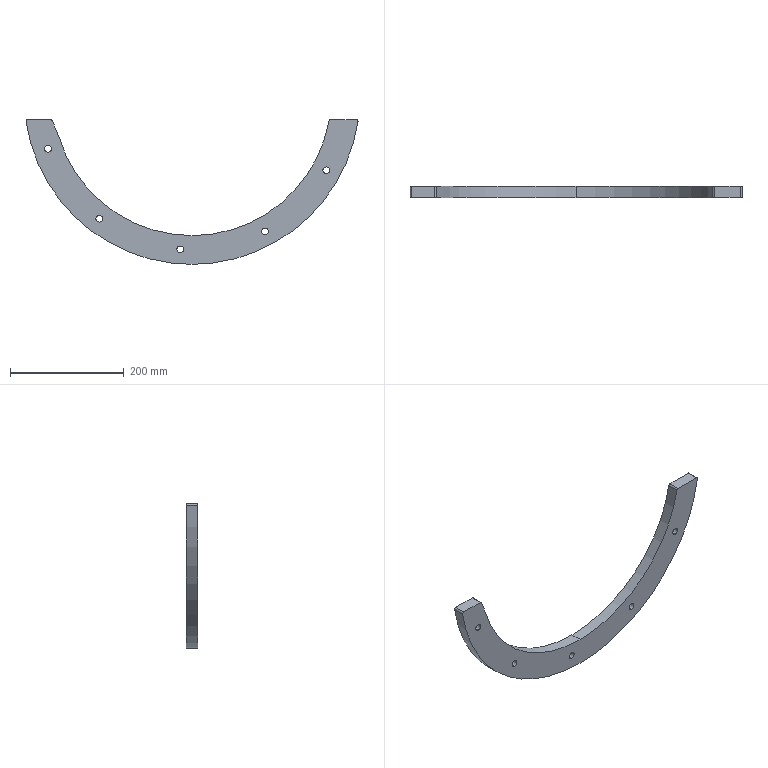Part | SolidWorks | features BaseBody 1 | 1 solid | 23 faces | box 584.886 x 20 x 255 mm | volume 765940 mm3 | cylinder 18 | plane 5 | commonest cylinder face diameters 12 x10 6 x4 490 x2 591.455 x2
STEP:
#1=CARTESIAN_POINT('',(-292.409,20.,-44.175));
#2=VERTEX_POINT('',#1);
#3=CARTESIAN_POINT('',(0.,20.,-295.727));
#4=VERTEX_POINT('',#3);
#5=CARTESIAN_POINT('',(0.,20.,0.));
#6=DIRECTION('',(0.,-1.,0.));
#7=DIRECTION('',(0.,0.,-1.));
#8=AXIS2_PLACEMENT_3D('',#5,#6,#7);
#9=CIRCLE('',#8,295.727);
#10=EDGE_CURVE('',#2,#4,#9,.T.);
#11=ORIENTED_EDGE('',*,*,#10,.T.);
#12=CARTESIAN_POINT('',(0.,0.,-295.727));
#13=VERTEX_POINT('',#12);
#14=CARTESIAN_POINT('',(0.,20.,-295.727));
#15=DIRECTION('',(0.,-1.,0.));
#16=VECTOR('',#15,1000.);
#17=LINE('',#14,#16);
#18=EDGE_CURVE('',#4,#13,#17,.T.);
#19=ORIENTED_EDGE('',*,*,#18,.T.);
#20=CARTESIAN_POINT('',(-292.409,0.,-44.175));
#21=VERTEX_POINT('',#20);
#22=CARTESIAN_POINT('',(0.,0.,0.));
#23=DIRECTION('',(0.,1.,0.));
#24=DIRECTION('',(0.,0.,-1.));
#25=AXIS2_PLACEMENT_3D('',#22,#23,#24);
#26=CIRCLE('',#25,295.727);
#27=EDGE_CURVE('',#13,#21,#26,.T.);
#28=ORIENTED_EDGE('',*,*,#27,.T.);
#29=CARTESIAN_POINT('',(-292.409,20.,-44.175));
#30=DIRECTION('',(0.,-1.,0.));
#31=VECTOR('',#30,1000.);
#32=LINE('',#29,#31);
#33=EDGE_CURVE('',#2,#21,#32,.T.);
#34=ORIENTED_EDGE('',*,*,#33,.F.);
#35=EDGE_LOOP('',(#11,#19,#28,#34));
#36=FACE_OUTER_BOUND('',#35,.T.);
#37=CARTESIAN_POINT('',(0.,20.,0.));
#38=DIRECTION('',(0.,-1.,0.));
#39=DIRECTION('',(0.,0.,-1.));
#40=AXIS2_PLACEMENT_3D('',#37,#38,#39);
#41=CYLINDRICAL_SURFACE('',#40,295.727);
#42=ADVANCED_FACE('',(#36),#41,.T.);
#43=CARTESIAN_POINT('',(0.,20.,-245.));
#44=VERTEX_POINT('',#43);
#45=CARTESIAN_POINT('',(241.162,20.,-43.198));
#46=VERTEX_POINT('',#45);
#47=CARTESIAN_POINT('',(0.,20.,0.));
#48=DIRECTION('',(0.,-1.,0.));
#49=DIRECTION('',(0.,0.,-1.));
#50=AXIS2_PLACEMENT_3D('',#47,#48,#49);
#51=CIRCLE('',#50,245.);
#52=EDGE_CURVE('',#44,#46,#51,.T.);
#53=ORIENTED_EDGE('',*,*,#52,.F.);
#54=CARTESIAN_POINT('',(0.,0.,-245.));
#55=VERTEX_POINT('',#54);
#56=CARTESIAN_POINT('',(0.,20.,-245.));
#57=DIRECTION('',(0.,-1.,0.));
#58=VECTOR('',#57,1000.);
#59=LINE('',#56,#58);
#60=EDGE_CURVE('',#44,#55,#59,.T.);
#61=ORIENTED_EDGE('',*,*,#60,.T.);
#62=CARTESIAN_POINT('',(241.162,0.,-43.198));
#63=VERTEX_POINT('',#62);
#64=CARTESIAN_POINT('',(0.,0.,0.));
#65=DIRECTION('',(0.,-1.,0.));
#66=DIRECTION('',(0.,0.,-1.));
#67=AXIS2_PLACEMENT_3D('',#64,#65,#66);
#68=CIRCLE('',#67,245.);
#69=EDGE_CURVE('',#55,#63,#68,.T.);
#70=ORIENTED_EDGE('',*,*,#69,.T.);
#71=CARTESIAN_POINT('',(241.162,20.,-43.198));
#72=DIRECTION('',(0.,-1.,0.));
#73=VECTOR('',#72,1000.);
#74=LINE('',#71,#73);
#75=EDGE_CURVE('',#46,#63,#74,.T.);
#76=ORIENTED_EDGE('',*,*,#75,.F.);
#77=EDGE_LOOP('',(#53,#61,#70,#76));
#78=FACE_OUTER_BOUND('',#77,.T.);
#79=CARTESIAN_POINT('',(0.,20.,0.));
#80=DIRECTION('',(0.,-1.,0.));
#81=DIRECTION('',(0.,0.,-1.));
#82=AXIS2_PLACEMENT_3D('',#79,#80,#81);
#83=CYLINDRICAL_SURFACE('',#82,245.);
#84=ADVANCED_FACE('',(#78),#83,.F.);
#85=CARTESIAN_POINT('',(-253.717,0.,-86.345));
#86=VERTEX_POINT('',#85);
#87=CARTESIAN_POINT('',(-253.717,0.,-98.345));
#88=VERTEX_POINT('',#87);
#89=CARTESIAN_POINT('',(-253.717,0.,-92.345));
#90=DIRECTION('',(0.,-1.,0.));
#91=DIRECTION('',(0.,0.,1.));
#92=AXIS2_PLACEMENT_3D('',#89,#90,#91);
#93=CIRCLE('',#92,6.);
#94=EDGE_CURVE('',#86,#88,#93,.T.);
#95=ORIENTED_EDGE('',*,*,#94,.T.);
#96=CARTESIAN_POINT('',(-253.717,20.,-98.345));
#97=VERTEX_POINT('',#96);
#98=CARTESIAN_POINT('',(-253.717,20.,-98.345));
#99=DIRECTION('',(0.,1.,0.));
#100=VECTOR('',#99,1000.);
#101=LINE('',#98,#100);
#102=EDGE_CURVE('',#88,#97,#101,.T.);
#103=ORIENTED_EDGE('',*,*,#102,.T.);
#104=CARTESIAN_POINT('',(-253.717,20.,-86.345));
#105=VERTEX_POINT('',#104);
#106=CARTESIAN_POINT('',(-253.717,20.,-92.345));
#107=DIRECTION('',(0.,-1.,0.));
#108=DIRECTION('',(0.,0.,1.));
#109=AXIS2_PLACEMENT_3D('',#106,#107,#108);
#110=CIRCLE('',#109,6.);
#111=EDGE_CURVE('',#105,#97,#110,.T.);
#112=ORIENTED_EDGE('',*,*,#111,.F.);
#113=CARTESIAN_POINT('',(-253.717,20.,-86.345));
#114=DIRECTION('',(0.,1.,0.));
#115=VECTOR('',#114,1000.);
#116=LINE('',#113,#115);
#117=EDGE_CURVE('',#86,#105,#116,.T.);
#118=ORIENTED_EDGE('',*,*,#117,.F.);
#119=EDGE_LOOP('',(#95,#103,#112,#118));
#120=FACE_OUTER_BOUND('',#119,.T.);
#121=CARTESIAN_POINT('',(-253.717,20.,-92.345));
#122=DIRECTION('',(0.,1.,0.));
#123=DIRECTION('',(0.,0.,1.));
#124=AXIS2_PLACEMENT_3D('',#121,#122,#123);
#125=CYLINDRICAL_SURFACE('',#124,6.);
#126=ADVANCED_FACE('',(#120),#125,.F.);
#127=CARTESIAN_POINT('',(236.708,0.,-124.148));
#128=VERTEX_POINT('',#127);
#129=CARTESIAN_POINT('',(236.708,0.,-136.148));
#130=VERTEX_POINT('',#129);
#131=CARTESIAN_POINT('',(236.708,0.,-130.148));
#132=DIRECTION('',(0.,-1.,0.));
#133=DIRECTION('',(0.,0.,1.));
#134=AXIS2_PLACEMENT_3D('',#131,#132,#133);
#135=CIRCLE('',#134,6.);
#136=EDGE_CURVE('',#128,#130,#135,.T.);
#137=ORIENTED_EDGE('',*,*,#136,.T.);
#138=CARTESIAN_POINT('',(236.708,20.,-136.148));
#139=VERTEX_POINT('',#138);
#140=CARTESIAN_POINT('',(236.708,20.,-136.148));
#141=DIRECTION('',(0.,1.,0.));
#142=VECTOR('',#141,1000.);
#143=LINE('',#140,#142);
#144=EDGE_CURVE('',#130,#139,#143,.T.);
#145=ORIENTED_EDGE('',*,*,#144,.T.);
#146=CARTESIAN_POINT('',(236.708,20.,-124.148));
#147=VERTEX_POINT('',#146);
#148=CARTESIAN_POINT('',(236.708,20.,-130.148));
#149=DIRECTION('',(0.,-1.,0.));
#150=DIRECTION('',(0.,0.,1.));
#151=AXIS2_PLACEMENT_3D('',#148,#149,#150);
#152=CIRCLE('',#151,6.);
#153=EDGE_CURVE('',#147,#139,#152,.T.);
#154=ORIENTED_EDGE('',*,*,#153,.F.);
#155=CARTESIAN_POINT('',(236.708,20.,-124.148));
#156=DIRECTION('',(0.,1.,0.));
#157=VECTOR('',#156,1000.);
#158=LINE('',#155,#157);
#159=EDGE_CURVE('',#128,#147,#158,.T.);
#160=ORIENTED_EDGE('',*,*,#159,.F.);
#161=EDGE_LOOP('',(#137,#145,#154,#160));
#162=FACE_OUTER_BOUND('',#161,.T.);
#163=CARTESIAN_POINT('',(236.708,20.,-130.148));
#164=DIRECTION('',(0.,1.,0.));
#165=DIRECTION('',(0.,0.,1.));
#166=AXIS2_PLACEMENT_3D('',#163,#164,#165);
#167=CYLINDRICAL_SURFACE('',#166,6.);
#168=ADVANCED_FACE('',(#162),#167,.F.);
#169=CARTESIAN_POINT('',(128.503,0.,-231.651));
#170=VERTEX_POINT('',#169);
#171=CARTESIAN_POINT('',(128.503,0.,-243.651));
#172=VERTEX_POINT('',#171);
#173=CARTESIAN_POINT('',(128.503,0.,-237.651));
#174=DIRECTION('',(0.,-1.,0.));
#175=DIRECTION('',(0.,0.,1.));
#176=AXIS2_PLACEMENT_3D('',#173,#174,#175);
#177=CIRCLE('',#176,6.);
#178=EDGE_CURVE('',#170,#172,#177,.T.);
#179=ORIENTED_EDGE('',*,*,#178,.T.);
#180=CARTESIAN_POINT('',(128.503,20.,-243.651));
#181=VERTEX_POINT('',#180);
#182=CARTESIAN_POINT('',(128.503,20.,-243.651));
#183=DIRECTION('',(0.,1.,0.));
#184=VECTOR('',#183,1000.);
#185=LINE('',#182,#184);
#186=EDGE_CURVE('',#172,#181,#185,.T.);
#187=ORIENTED_EDGE('',*,*,#186,.T.);
#188=CARTESIAN_POINT('',(128.503,20.,-231.651));
#189=VERTEX_POINT('',#188);
#190=CARTESIAN_POINT('',(128.503,20.,-237.651));
#191=DIRECTION('',(0.,-1.,0.));
#192=DIRECTION('',(0.,0.,1.));
#193=AXIS2_PLACEMENT_3D('',#190,#191,#192);
#194=CIRCLE('',#193,6.);
#195=EDGE_CURVE('',#189,#181,#194,.T.);
#196=ORIENTED_EDGE('',*,*,#195,.F.);
#197=CARTESIAN_POINT('',(128.503,20.,-231.651));
#198=DIRECTION('',(0.,1.,0.));
#199=VECTOR('',#198,1000.);
#200=LINE('',#197,#199);
#201=EDGE_CURVE('',#170,#189,#200,.T.);
#202=ORIENTED_EDGE('',*,*,#201,.F.);
#203=EDGE_LOOP('',(#179,#187,#196,#202));
#204=FACE_OUTER_BOUND('',#203,.T.);
#205=CARTESIAN_POINT('',(128.503,20.,-237.651));
#206=DIRECTION('',(0.,1.,0.));
#207=DIRECTION('',(0.,0.,1.));
#208=AXIS2_PLACEMENT_3D('',#205,#206,#207);
#209=CYLINDRICAL_SURFACE('',#208,6.);
#210=ADVANCED_FACE('',(#204),#209,.F.);
#211=CARTESIAN_POINT('',(-20.692,0.,-263.361));
#212=VERTEX_POINT('',#211);
#213=CARTESIAN_POINT('',(-20.692,0.,-275.361));
#214=VERTEX_POINT('',#213);
#215=CARTESIAN_POINT('',(-20.692,0.,-269.361));
#216=DIRECTION('',(0.,-1.,0.));
#217=DIRECTION('',(0.,0.,1.));
#218=AXIS2_PLACEMENT_3D('',#215,#216,#217);
#219=CIRCLE('',#218,6.);
#220=EDGE_CURVE('',#212,#214,#219,.T.);
#221=ORIENTED_EDGE('',*,*,#220,.T.);
#222=CARTESIAN_POINT('',(-20.692,20.,-275.361));
#223=VERTEX_POINT('',#222);
#224=CARTESIAN_POINT('',(-20.692,20.,-275.361));
#225=DIRECTION('',(0.,1.,0.));
#226=VECTOR('',#225,1000.);
#227=LINE('',#224,#226);
#228=EDGE_CURVE('',#214,#223,#227,.T.);
#229=ORIENTED_EDGE('',*,*,#228,.T.);
#230=CARTESIAN_POINT('',(-20.692,20.,-263.361));
#231=VERTEX_POINT('',#230);
#232=CARTESIAN_POINT('',(-20.692,20.,-269.361));
#233=DIRECTION('',(0.,-1.,0.));
#234=DIRECTION('',(0.,0.,1.));
#235=AXIS2_PLACEMENT_3D('',#232,#233,#234);
#236=CIRCLE('',#235,6.);
#237=EDGE_CURVE('',#231,#223,#236,.T.);
#238=ORIENTED_EDGE('',*,*,#237,.F.);
#239=CARTESIAN_POINT('',(-20.692,20.,-263.361));
#240=DIRECTION('',(0.,1.,0.));
#241=VECTOR('',#240,1000.);
#242=LINE('',#239,#241);
#243=EDGE_CURVE('',#212,#231,#242,.T.);
#244=ORIENTED_EDGE('',*,*,#243,.F.);
#245=EDGE_LOOP('',(#221,#229,#238,#244));
#246=FACE_OUTER_BOUND('',#245,.T.);
#247=CARTESIAN_POINT('',(-20.692,20.,-269.361));
#248=DIRECTION('',(0.,1.,0.));
#249=DIRECTION('',(0.,0.,1.));
#250=AXIS2_PLACEMENT_3D('',#247,#248,#249);
#251=CYLINDRICAL_SURFACE('',#250,6.);
#252=ADVANCED_FACE('',(#246),#251,.F.);
#253=CARTESIAN_POINT('',(-163.266,0.,-209.161));
#254=VERTEX_POINT('',#253);
#255=CARTESIAN_POINT('',(-163.266,0.,-221.161));
#256=VERTEX_POINT('',#255);
#257=CARTESIAN_POINT('',(-163.266,0.,-215.161));
#258=DIRECTION('',(0.,-1.,0.));
#259=DIRECTION('',(0.,0.,1.));
#260=AXIS2_PLACEMENT_3D('',#257,#258,#259);
#261=CIRCLE('',#260,6.);
#262=EDGE_CURVE('',#254,#256,#261,.T.);
#263=ORIENTED_EDGE('',*,*,#262,.T.);
#264=CARTESIAN_POINT('',(-163.266,20.,-221.161));
#265=VERTEX_POINT('',#264);
#266=CARTESIAN_POINT('',(-163.266,20.,-221.161));
#267=DIRECTION('',(0.,1.,0.));
#268=VECTOR('',#267,1000.);
#269=LINE('',#266,#268);
#270=EDGE_CURVE('',#256,#265,#269,.T.);
#271=ORIENTED_EDGE('',*,*,#270,.T.);
#272=CARTESIAN_POINT('',(-163.266,20.,-209.161));
#273=VERTEX_POINT('',#272);
#274=CARTESIAN_POINT('',(-163.266,20.,-215.161));
#275=DIRECTION('',(0.,-1.,0.));
#276=DIRECTION('',(0.,0.,1.));
#277=AXIS2_PLACEMENT_3D('',#274,#275,#276);
#278=CIRCLE('',#277,6.);
#279=EDGE_CURVE('',#273,#265,#278,.T.);
#280=ORIENTED_EDGE('',*,*,#279,.F.);
#281=CARTESIAN_POINT('',(-163.266,20.,-209.161));
#282=DIRECTION('',(0.,1.,0.));
#283=VECTOR('',#282,1000.);
#284=LINE('',#281,#283);
#285=EDGE_CURVE('',#254,#273,#284,.T.);
#286=ORIENTED_EDGE('',*,*,#285,.F.);
#287=EDGE_LOOP('',(#263,#271,#280,#286));
#288=FACE_OUTER_BOUND('',#287,.T.);
#289=CARTESIAN_POINT('',(-163.266,20.,-215.161));
#290=DIRECTION('',(0.,1.,0.));
#291=DIRECTION('',(0.,0.,1.));
#292=AXIS2_PLACEMENT_3D('',#289,#290,#291);
#293=CYLINDRICAL_SURFACE('',#292,6.);
#294=ADVANCED_FACE('',(#288),#293,.F.);
#295=CARTESIAN_POINT('',(289.443,0.,-40.727));
#296=VERTEX_POINT('',#295);
#297=CARTESIAN_POINT('',(292.409,0.,-44.175));
#298=VERTEX_POINT('',#297);
#299=CARTESIAN_POINT('',(289.443,0.,-43.727));
#300=DIRECTION('',(0.,1.,0.));
#301=DIRECTION('',(0.,0.,-1.));
#302=AXIS2_PLACEMENT_3D('',#299,#300,#301);
#303=CIRCLE('',#302,3.);
#304=EDGE_CURVE('',#296,#298,#303,.T.);
#305=ORIENTED_EDGE('',*,*,#304,.F.);
#306=CARTESIAN_POINT('',(244.115,0.,-40.727));
#307=VERTEX_POINT('',#306);
#308=CARTESIAN_POINT('',(0.,0.,-40.727));
#309=DIRECTION('',(1.,0.,0.));
#310=VECTOR('',#309,1000.);
#311=LINE('',#308,#310);
#312=EDGE_CURVE('',#307,#296,#311,.T.);
#313=ORIENTED_EDGE('',*,*,#312,.F.);
#314=CARTESIAN_POINT('',(244.115,0.,-43.727));
#315=DIRECTION('',(0.,1.,0.));
#316=DIRECTION('',(0.,0.,-1.));
#317=AXIS2_PLACEMENT_3D('',#314,#315,#316);
#318=CIRCLE('',#317,3.);
#319=EDGE_CURVE('',#63,#307,#318,.T.);
#320=ORIENTED_EDGE('',*,*,#319,.F.);
#321=ORIENTED_EDGE('',*,*,#69,.F.);
#322=CARTESIAN_POINT('',(-234.569,0.,-70.727));
#323=VERTEX_POINT('',#322);
#324=CARTESIAN_POINT('',(0.,0.,0.));
#325=DIRECTION('',(0.,-1.,0.));
#326=DIRECTION('',(0.,0.,-1.));
#327=AXIS2_PLACEMENT_3D('',#324,#325,#326);
#328=CIRCLE('',#327,245.);
#329=EDGE_CURVE('',#323,#55,#328,.T.);
#330=ORIENTED_EDGE('',*,*,#329,.F.);
#331=CARTESIAN_POINT('',(-246.065,0.,-42.592));
#332=VERTEX_POINT('',#331);
#333=CARTESIAN_POINT('',(-246.065,0.,-42.592));
#334=DIRECTION('',(0.3783,0.,-0.9257));
#335=VECTOR('',#334,1000.);
#336=LINE('',#333,#335);
#337=EDGE_CURVE('',#332,#323,#336,.T.);
#338=ORIENTED_EDGE('',*,*,#337,.F.);
#339=CARTESIAN_POINT('',(-248.843,0.,-40.727));
#340=VERTEX_POINT('',#339);
#341=CARTESIAN_POINT('',(-248.843,0.,-43.727));
#342=DIRECTION('',(0.,1.,0.));
#343=DIRECTION('',(0.,0.,-1.));
#344=AXIS2_PLACEMENT_3D('',#341,#342,#343);
#345=CIRCLE('',#344,3.);
#346=EDGE_CURVE('',#340,#332,#345,.T.);
#347=ORIENTED_EDGE('',*,*,#346,.F.);
#348=CARTESIAN_POINT('',(-289.443,0.,-40.727));
#349=VERTEX_POINT('',#348);
#350=CARTESIAN_POINT('',(0.,0.,-40.727));
#351=DIRECTION('',(1.,0.,0.));
#352=VECTOR('',#351,1000.);
#353=LINE('',#350,#352);
#354=EDGE_CURVE('',#349,#340,#353,.T.);
#355=ORIENTED_EDGE('',*,*,#354,.F.);
#356=CARTESIAN_POINT('',(-289.443,0.,-43.727));
#357=DIRECTION('',(0.,1.,0.));
#358=DIRECTION('',(0.,0.,-1.));
#359=AXIS2_PLACEMENT_3D('',#356,#357,#358);
#360=CIRCLE('',#359,3.);
#361=EDGE_CURVE('',#21,#349,#360,.T.);
#362=ORIENTED_EDGE('',*,*,#361,.F.);
#363=ORIENTED_EDGE('',*,*,#27,.F.);
#364=CARTESIAN_POINT('',(0.,0.,0.));
#365=DIRECTION('',(0.,1.,0.));
#366=DIRECTION('',(0.,0.,-1.));
#367=AXIS2_PLACEMENT_3D('',#364,#365,#366);
#368=CIRCLE('',#367,295.727);
#369=EDGE_CURVE('',#298,#13,#368,.T.);
#370=ORIENTED_EDGE('',*,*,#369,.F.);
#371=EDGE_LOOP('',(#305,#313,#320,#321,#330,#338,#347,#355,#362,#363,#370));
#372=FACE_OUTER_BOUND('',#371,.T.);
#373=ORIENTED_EDGE('',*,*,#94,.F.);
#374=CARTESIAN_POINT('',(-253.717,0.,-92.345));
#375=DIRECTION('',(0.,-1.,0.));
#376=DIRECTION('',(0.,0.,1.));
#377=AXIS2_PLACEMENT_3D('',#374,#375,#376);
#378=CIRCLE('',#377,6.);
#379=EDGE_CURVE('',#88,#86,#378,.T.);
#380=ORIENTED_EDGE('',*,*,#379,.F.);
#381=EDGE_LOOP('',(#373,#380));
#382=FACE_BOUND('',#381,.T.);
#383=ORIENTED_EDGE('',*,*,#136,.F.);
#384=CARTESIAN_POINT('',(236.708,0.,-130.148));
#385=DIRECTION('',(0.,-1.,0.));
#386=DIRECTION('',(0.,0.,1.));
#387=AXIS2_PLACEMENT_3D('',#384,#385,#386);
#388=CIRCLE('',#387,6.);
#389=EDGE_CURVE('',#130,#128,#388,.T.);
#390=ORIENTED_EDGE('',*,*,#389,.F.);
#391=EDGE_LOOP('',(#383,#390));
#392=FACE_BOUND('',#391,.T.);
#393=ORIENTED_EDGE('',*,*,#178,.F.);
#394=CARTESIAN_POINT('',(128.503,0.,-237.651));
#395=DIRECTION('',(0.,-1.,0.));
#396=DIRECTION('',(0.,0.,1.));
#397=AXIS2_PLACEMENT_3D('',#394,#395,#396);
#398=CIRCLE('',#397,6.);
#399=EDGE_CURVE('',#172,#170,#398,.T.);
#400=ORIENTED_EDGE('',*,*,#399,.F.);
#401=EDGE_LOOP('',(#393,#400));
#402=FACE_BOUND('',#401,.T.);
#403=ORIENTED_EDGE('',*,*,#220,.F.);
#404=CARTESIAN_POINT('',(-20.692,0.,-269.361));
#405=DIRECTION('',(0.,-1.,0.));
#406=DIRECTION('',(0.,0.,1.));
#407=AXIS2_PLACEMENT_3D('',#404,#405,#406);
#408=CIRCLE('',#407,6.);
#409=EDGE_CURVE('',#214,#212,#408,.T.);
#410=ORIENTED_EDGE('',*,*,#409,.F.);
#411=EDGE_LOOP('',(#403,#410));
#412=FACE_BOUND('',#411,.T.);
#413=ORIENTED_EDGE('',*,*,#262,.F.);
#414=CARTESIAN_POINT('',(-163.266,0.,-215.161));
#415=DIRECTION('',(0.,-1.,0.));
#416=DIRECTION('',(0.,0.,1.));
#417=AXIS2_PLACEMENT_3D('',#414,#415,#416);
#418=CIRCLE('',#417,6.);
#419=EDGE_CURVE('',#256,#254,#418,.T.);
#420=ORIENTED_EDGE('',*,*,#419,.F.);
#421=EDGE_LOOP('',(#413,#420));
#422=FACE_BOUND('',#421,.T.);
#423=CARTESIAN_POINT('',(0.,0.,0.));
#424=DIRECTION('',(0.,1.,0.));
#425=DIRECTION('',(0.,0.,1.));
#426=AXIS2_PLACEMENT_3D('',#423,#424,#425);
#427=PLANE('',#426);
#428=ADVANCED_FACE('',(#372,#382,#392,#402,#412,#422),#427,.F.);
#429=ORIENTED_EDGE('',*,*,#18,.F.);
#430=CARTESIAN_POINT('',(292.409,20.,-44.175));
#431=VERTEX_POINT('',#430);
#432=CARTESIAN_POINT('',(0.,20.,0.));
#433=DIRECTION('',(0.,-1.,0.));
#434=DIRECTION('',(0.,0.,-1.));
#435=AXIS2_PLACEMENT_3D('',#432,#433,#434);
#436=CIRCLE('',#435,295.727);
#437=EDGE_CURVE('',#4,#431,#436,.T.);
#438=ORIENTED_EDGE('',*,*,#437,.T.);
#439=CARTESIAN_POINT('',(292.409,20.,-44.175));
#440=DIRECTION('',(0.,-1.,0.));
#441=VECTOR('',#440,1000.);
#442=LINE('',#439,#441);
#443=EDGE_CURVE('',#431,#298,#442,.T.);
#444=ORIENTED_EDGE('',*,*,#443,.T.);
#445=ORIENTED_EDGE('',*,*,#369,.T.);
#446=EDGE_LOOP('',(#429,#438,#444,#445));
#447=FACE_OUTER_BOUND('',#446,.T.);
#448=CARTESIAN_POINT('',(0.,20.,0.));
#449=DIRECTION('',(0.,-1.,0.));
#450=DIRECTION('',(0.,0.,-1.));
#451=AXIS2_PLACEMENT_3D('',#448,#449,#450);
#452=CYLINDRICAL_SURFACE('',#451,295.727);
#453=ADVANCED_FACE('',(#447),#452,.T.);
#454=ORIENTED_EDGE('',*,*,#304,.T.);
#455=ORIENTED_EDGE('',*,*,#443,.F.);
#456=CARTESIAN_POINT('',(289.443,20.,-40.727));
#457=VERTEX_POINT('',#456);
#458=CARTESIAN_POINT('',(289.443,20.,-43.727));
#459=DIRECTION('',(0.,-1.,0.));
#460=DIRECTION('',(0.,0.,-1.));
#461=AXIS2_PLACEMENT_3D('',#458,#459,#460);
#462=CIRCLE('',#461,3.);
#463=EDGE_CURVE('',#431,#457,#462,.T.);
#464=ORIENTED_EDGE('',*,*,#463,.T.);
#465=CARTESIAN_POINT('',(289.443,20.,-40.727));
#466=DIRECTION('',(0.,-1.,0.));
#467=VECTOR('',#466,1000.);
#468=LINE('',#465,#467);
#469=EDGE_CURVE('',#457,#296,#468,.T.);
#470=ORIENTED_EDGE('',*,*,#469,.T.);
#471=EDGE_LOOP('',(#454,#455,#464,#470));
#472=FACE_OUTER_BOUND('',#471,.T.);
#473=CARTESIAN_POINT('',(289.443,20.,-43.727));
#474=DIRECTION('',(0.,-1.,0.));
#475=DIRECTION('',(0.,0.,-1.));
#476=AXIS2_PLACEMENT_3D('',#473,#474,#475);
#477=CYLINDRICAL_SURFACE('',#476,3.);
#478=ADVANCED_FACE('',(#472),#477,.T.);
#479=ORIENTED_EDGE('',*,*,#469,.F.);
#480=CARTESIAN_POINT('',(244.115,20.,-40.727));
#481=VERTEX_POINT('',#480);
#482=CARTESIAN_POINT('',(-346.299,20.,-40.727));
#483=DIRECTION('',(1.,0.,0.));
#484=VECTOR('',#483,1000.);
#485=LINE('',#482,#484);
#486=EDGE_CURVE('',#481,#457,#485,.T.);
#487=ORIENTED_EDGE('',*,*,#486,.F.);
#488=CARTESIAN_POINT('',(244.115,0.,-40.727));
#489=DIRECTION('',(0.,1.,0.));
#490=VECTOR('',#489,1000.);
#491=LINE('',#488,#490);
#492=EDGE_CURVE('',#307,#481,#491,.T.);
#493=ORIENTED_EDGE('',*,*,#492,.F.);
#494=ORIENTED_EDGE('',*,*,#312,.T.);
#495=EDGE_LOOP('',(#479,#487,#493,#494));
#496=FACE_OUTER_BOUND('',#495,.T.);
#497=CARTESIAN_POINT('',(-346.299,0.,-40.727));
#498=DIRECTION('',(0.,0.,-1.));
#499=DIRECTION('',(-1.,0.,0.));
#500=AXIS2_PLACEMENT_3D('',#497,#498,#499);
#501=PLANE('',#500);
#502=ADVANCED_FACE('',(#496),#501,.F.);
#503=CARTESIAN_POINT('',(244.115,20.,-43.727));
#504=DIRECTION('',(0.,-1.,0.));
#505=DIRECTION('',(0.,0.,-1.));
#506=AXIS2_PLACEMENT_3D('',#503,#504,#505);
#507=CIRCLE('',#506,3.);
#508=EDGE_CURVE('',#481,#46,#507,.T.);
#509=ORIENTED_EDGE('',*,*,#508,.T.);
#510=ORIENTED_EDGE('',*,*,#75,.T.);
#511=ORIENTED_EDGE('',*,*,#319,.T.);
#512=ORIENTED_EDGE('',*,*,#492,.T.);
#513=EDGE_LOOP('',(#509,#510,#511,#512));
#514=FACE_OUTER_BOUND('',#513,.T.);
#515=CARTESIAN_POINT('',(244.115,20.,-43.727));
#516=DIRECTION('',(0.,-1.,0.));
#517=DIRECTION('',(0.,0.,-1.));
#518=AXIS2_PLACEMENT_3D('',#515,#516,#517);
#519=CYLINDRICAL_SURFACE('',#518,3.);
#520=ADVANCED_FACE('',(#514),#519,.T.);
#521=ORIENTED_EDGE('',*,*,#60,.F.);
#522=CARTESIAN_POINT('',(-234.569,20.,-70.727));
#523=VERTEX_POINT('',#522);
#524=CARTESIAN_POINT('',(0.,20.,0.));
#525=DIRECTION('',(0.,-1.,0.));
#526=DIRECTION('',(0.,0.,-1.));
#527=AXIS2_PLACEMENT_3D('',#524,#525,#526);
#528=CIRCLE('',#527,245.);
#529=EDGE_CURVE('',#523,#44,#528,.T.);
#530=ORIENTED_EDGE('',*,*,#529,.F.);
#531=CARTESIAN_POINT('',(-234.569,20.,-70.727));
#532=DIRECTION('',(0.,1.,0.));
#533=VECTOR('',#532,1000.);
#534=LINE('',#531,#533);
#535=EDGE_CURVE('',#323,#523,#534,.T.);
#536=ORIENTED_EDGE('',*,*,#535,.F.);
#537=ORIENTED_EDGE('',*,*,#329,.T.);
#538=EDGE_LOOP('',(#521,#530,#536,#537));
#539=FACE_OUTER_BOUND('',#538,.T.);
#540=CARTESIAN_POINT('',(0.,20.,0.));
#541=DIRECTION('',(0.,-1.,0.));
#542=DIRECTION('',(0.,0.,-1.));
#543=AXIS2_PLACEMENT_3D('',#540,#541,#542);
#544=CYLINDRICAL_SURFACE('',#543,245.);
#545=ADVANCED_FACE('',(#539),#544,.F.);
#546=CARTESIAN_POINT('',(-246.065,20.,-42.592));
#547=VERTEX_POINT('',#546);
#548=CARTESIAN_POINT('',(-246.065,0.,-42.592));
#549=DIRECTION('',(0.,1.,0.));
#550=VECTOR('',#549,1000.);
#551=LINE('',#548,#550);
#552=EDGE_CURVE('',#332,#547,#551,.T.);
#553=ORIENTED_EDGE('',*,*,#552,.F.);
#554=ORIENTED_EDGE('',*,*,#337,.T.);
#555=ORIENTED_EDGE('',*,*,#535,.T.);
#556=CARTESIAN_POINT('',(-255.,20.,-20.727));
#557=DIRECTION('',(0.3783,0.,-0.9257));
#558=VECTOR('',#557,1000.);
#559=LINE('',#556,#558);
#560=EDGE_CURVE('',#547,#523,#559,.T.);
#561=ORIENTED_EDGE('',*,*,#560,.F.);
#562=EDGE_LOOP('',(#553,#554,#555,#561));
#563=FACE_OUTER_BOUND('',#562,.T.);
#564=CARTESIAN_POINT('',(-255.,0.,-20.727));
#565=DIRECTION('',(-0.9257,0.,-0.3783));
#566=DIRECTION('',(-0.3783,0.,0.9257));
#567=AXIS2_PLACEMENT_3D('',#564,#565,#566);
#568=PLANE('',#567);
#569=ADVANCED_FACE('',(#563),#568,.F.);
#570=ORIENTED_EDGE('',*,*,#346,.T.);
#571=ORIENTED_EDGE('',*,*,#552,.T.);
#572=CARTESIAN_POINT('',(-248.843,20.,-40.727));
#573=VERTEX_POINT('',#572);
#574=CARTESIAN_POINT('',(-248.843,20.,-43.727));
#575=DIRECTION('',(0.,-1.,0.));
#576=DIRECTION('',(0.,0.,-1.));
#577=AXIS2_PLACEMENT_3D('',#574,#575,#576);
#578=CIRCLE('',#577,3.);
#579=EDGE_CURVE('',#547,#573,#578,.T.);
#580=ORIENTED_EDGE('',*,*,#579,.T.);
#581=CARTESIAN_POINT('',(-248.843,0.,-40.727));
#582=DIRECTION('',(0.,-1.,0.));
#583=VECTOR('',#582,1000.);
#584=LINE('',#581,#583);
#585=EDGE_CURVE('',#573,#340,#584,.T.);
#586=ORIENTED_EDGE('',*,*,#585,.T.);
#587=EDGE_LOOP('',(#570,#571,#580,#586));
#588=FACE_OUTER_BOUND('',#587,.T.);
#589=CARTESIAN_POINT('',(-248.843,0.,-43.727));
#590=DIRECTION('',(0.,-1.,0.));
#591=DIRECTION('',(0.,0.,-1.));
#592=AXIS2_PLACEMENT_3D('',#589,#590,#591);
#593=CYLINDRICAL_SURFACE('',#592,3.);
#594=ADVANCED_FACE('',(#588),#593,.T.);
#595=ORIENTED_EDGE('',*,*,#585,.F.);
#596=CARTESIAN_POINT('',(-289.443,20.,-40.727));
#597=VERTEX_POINT('',#596);
#598=CARTESIAN_POINT('',(-346.299,20.,-40.727));
#599=DIRECTION('',(1.,0.,0.));
#600=VECTOR('',#599,1000.);
#601=LINE('',#598,#600);
#602=EDGE_CURVE('',#597,#573,#601,.T.);
#603=ORIENTED_EDGE('',*,*,#602,.F.);
#604=CARTESIAN_POINT('',(-289.443,0.,-40.727));
#605=DIRECTION('',(0.,1.,0.));
#606=VECTOR('',#605,1000.);
#607=LINE('',#604,#606);
#608=EDGE_CURVE('',#349,#597,#607,.T.);
#609=ORIENTED_EDGE('',*,*,#608,.F.);
#610=ORIENTED_EDGE('',*,*,#354,.T.);
#611=EDGE_LOOP('',(#595,#603,#609,#610));
#612=FACE_OUTER_BOUND('',#611,.T.);
#613=CARTESIAN_POINT('',(-346.299,0.,-40.727));
#614=DIRECTION('',(0.,0.,-1.));
#615=DIRECTION('',(-1.,0.,0.));
#616=AXIS2_PLACEMENT_3D('',#613,#614,#615);
#617=PLANE('',#616);
#618=ADVANCED_FACE('',(#612),#617,.F.);
#619=CARTESIAN_POINT('',(-289.443,20.,-43.727));
#620=DIRECTION('',(0.,-1.,0.));
#621=DIRECTION('',(0.,0.,-1.));
#622=AXIS2_PLACEMENT_3D('',#619,#620,#621);
#623=CIRCLE('',#622,3.);
#624=EDGE_CURVE('',#597,#2,#623,.T.);
#625=ORIENTED_EDGE('',*,*,#624,.T.);
#626=ORIENTED_EDGE('',*,*,#33,.T.);
#627=ORIENTED_EDGE('',*,*,#361,.T.);
#628=ORIENTED_EDGE('',*,*,#608,.T.);
#629=EDGE_LOOP('',(#625,#626,#627,#628));
#630=FACE_OUTER_BOUND('',#629,.T.);
#631=CARTESIAN_POINT('',(-289.443,20.,-43.727));
#632=DIRECTION('',(0.,-1.,0.));
#633=DIRECTION('',(0.,0.,-1.));
#634=AXIS2_PLACEMENT_3D('',#631,#632,#633);
#635=CYLINDRICAL_SURFACE('',#634,3.);
#636=ADVANCED_FACE('',(#630),#635,.T.);
#637=ORIENTED_EDGE('',*,*,#102,.F.);
#638=ORIENTED_EDGE('',*,*,#379,.T.);
#639=ORIENTED_EDGE('',*,*,#117,.T.);
#640=CARTESIAN_POINT('',(-253.717,20.,-92.345));
#641=DIRECTION('',(0.,-1.,0.));
#642=DIRECTION('',(0.,0.,1.));
#643=AXIS2_PLACEMENT_3D('',#640,#641,#642);
#644=CIRCLE('',#643,6.);
#645=EDGE_CURVE('',#97,#105,#644,.T.);
#646=ORIENTED_EDGE('',*,*,#645,.F.);
#647=EDGE_LOOP('',(#637,#638,#639,#646));
#648=FACE_OUTER_BOUND('',#647,.T.);
#649=CARTESIAN_POINT('',(-253.717,20.,-92.345));
#650=DIRECTION('',(0.,1.,0.));
#651=DIRECTION('',(0.,0.,1.));
#652=AXIS2_PLACEMENT_3D('',#649,#650,#651);
#653=CYLINDRICAL_SURFACE('',#652,6.);
#654=ADVANCED_FACE('',(#648),#653,.F.);
#655=ORIENTED_EDGE('',*,*,#144,.F.);
#656=ORIENTED_EDGE('',*,*,#389,.T.);
#657=ORIENTED_EDGE('',*,*,#159,.T.);
#658=CARTESIAN_POINT('',(236.708,20.,-130.148));
#659=DIRECTION('',(0.,-1.,0.));
#660=DIRECTION('',(0.,0.,1.));
#661=AXIS2_PLACEMENT_3D('',#658,#659,#660);
#662=CIRCLE('',#661,6.);
#663=EDGE_CURVE('',#139,#147,#662,.T.);
#664=ORIENTED_EDGE('',*,*,#663,.F.);
#665=EDGE_LOOP('',(#655,#656,#657,#664));
#666=FACE_OUTER_BOUND('',#665,.T.);
#667=CARTESIAN_POINT('',(236.708,20.,-130.148));
#668=DIRECTION('',(0.,1.,0.));
#669=DIRECTION('',(0.,0.,1.));
#670=AXIS2_PLACEMENT_3D('',#667,#668,#669);
#671=CYLINDRICAL_SURFACE('',#670,6.);
#672=ADVANCED_FACE('',(#666),#671,.F.);
#673=ORIENTED_EDGE('',*,*,#186,.F.);
#674=ORIENTED_EDGE('',*,*,#399,.T.);
#675=ORIENTED_EDGE('',*,*,#201,.T.);
#676=CARTESIAN_POINT('',(128.503,20.,-237.651));
#677=DIRECTION('',(0.,-1.,0.));
#678=DIRECTION('',(0.,0.,1.));
#679=AXIS2_PLACEMENT_3D('',#676,#677,#678);
#680=CIRCLE('',#679,6.);
#681=EDGE_CURVE('',#181,#189,#680,.T.);
#682=ORIENTED_EDGE('',*,*,#681,.F.);
#683=EDGE_LOOP('',(#673,#674,#675,#682));
#684=FACE_OUTER_BOUND('',#683,.T.);
#685=CARTESIAN_POINT('',(128.503,20.,-237.651));
#686=DIRECTION('',(0.,1.,0.));
#687=DIRECTION('',(0.,0.,1.));
#688=AXIS2_PLACEMENT_3D('',#685,#686,#687);
#689=CYLINDRICAL_SURFACE('',#688,6.);
#690=ADVANCED_FACE('',(#684),#689,.F.);
#691=ORIENTED_EDGE('',*,*,#228,.F.);
#692=ORIENTED_EDGE('',*,*,#409,.T.);
#693=ORIENTED_EDGE('',*,*,#243,.T.);
#694=CARTESIAN_POINT('',(-20.692,20.,-269.361));
#695=DIRECTION('',(0.,-1.,0.));
#696=DIRECTION('',(0.,0.,1.));
#697=AXIS2_PLACEMENT_3D('',#694,#695,#696);
#698=CIRCLE('',#697,6.);
#699=EDGE_CURVE('',#223,#231,#698,.T.);
#700=ORIENTED_EDGE('',*,*,#699,.F.);
#701=EDGE_LOOP('',(#691,#692,#693,#700));
#702=FACE_OUTER_BOUND('',#701,.T.);
#703=CARTESIAN_POINT('',(-20.692,20.,-269.361));
#704=DIRECTION('',(0.,1.,0.));
#705=DIRECTION('',(0.,0.,1.));
#706=AXIS2_PLACEMENT_3D('',#703,#704,#705);
#707=CYLINDRICAL_SURFACE('',#706,6.);
#708=ADVANCED_FACE('',(#702),#707,.F.);
#709=ORIENTED_EDGE('',*,*,#270,.F.);
#710=ORIENTED_EDGE('',*,*,#419,.T.);
#711=ORIENTED_EDGE('',*,*,#285,.T.);
#712=CARTESIAN_POINT('',(-163.266,20.,-215.161));
#713=DIRECTION('',(0.,-1.,0.));
#714=DIRECTION('',(0.,0.,1.));
#715=AXIS2_PLACEMENT_3D('',#712,#713,#714);
#716=CIRCLE('',#715,6.);
#717=EDGE_CURVE('',#265,#273,#716,.T.);
#718=ORIENTED_EDGE('',*,*,#717,.F.);
#719=EDGE_LOOP('',(#709,#710,#711,#718));
#720=FACE_OUTER_BOUND('',#719,.T.);
#721=CARTESIAN_POINT('',(-163.266,20.,-215.161));
#722=DIRECTION('',(0.,1.,0.));
#723=DIRECTION('',(0.,0.,1.));
#724=AXIS2_PLACEMENT_3D('',#721,#722,#723);
#725=CYLINDRICAL_SURFACE('',#724,6.);
#726=ADVANCED_FACE('',(#720),#725,.F.);
#727=ORIENTED_EDGE('',*,*,#111,.T.);
#728=ORIENTED_EDGE('',*,*,#645,.T.);
#729=EDGE_LOOP('',(#727,#728));
#730=FACE_BOUND('',#729,.T.);
#731=ORIENTED_EDGE('',*,*,#153,.T.);
#732=ORIENTED_EDGE('',*,*,#663,.T.);
#733=EDGE_LOOP('',(#731,#732));
#734=FACE_BOUND('',#733,.T.);
#735=ORIENTED_EDGE('',*,*,#195,.T.);
#736=ORIENTED_EDGE('',*,*,#681,.T.);
#737=EDGE_LOOP('',(#735,#736));
#738=FACE_BOUND('',#737,.T.);
#739=ORIENTED_EDGE('',*,*,#237,.T.);
#740=ORIENTED_EDGE('',*,*,#699,.T.);
#741=EDGE_LOOP('',(#739,#740));
#742=FACE_BOUND('',#741,.T.);
#743=ORIENTED_EDGE('',*,*,#279,.T.);
#744=ORIENTED_EDGE('',*,*,#717,.T.);
#745=EDGE_LOOP('',(#743,#744));
#746=FACE_BOUND('',#745,.T.);
#747=ORIENTED_EDGE('',*,*,#529,.T.);
#748=ORIENTED_EDGE('',*,*,#52,.T.);
#749=ORIENTED_EDGE('',*,*,#508,.F.);
#750=ORIENTED_EDGE('',*,*,#486,.T.);
#751=ORIENTED_EDGE('',*,*,#463,.F.);
#752=ORIENTED_EDGE('',*,*,#437,.F.);
#753=ORIENTED_EDGE('',*,*,#10,.F.);
#754=ORIENTED_EDGE('',*,*,#624,.F.);
#755=ORIENTED_EDGE('',*,*,#602,.T.);
#756=ORIENTED_EDGE('',*,*,#579,.F.);
#757=ORIENTED_EDGE('',*,*,#560,.T.);
#758=EDGE_LOOP('',(#747,#748,#749,#750,#751,#752,#753,#754,#755,#756,#757));
#759=FACE_OUTER_BOUND('',#758,.T.);
#760=CARTESIAN_POINT('',(0.,20.,0.));
#761=DIRECTION('',(0.,1.,0.));
#762=DIRECTION('',(0.,0.,1.));
#763=AXIS2_PLACEMENT_3D('',#760,#761,#762);
#764=PLANE('',#763);
#765=ADVANCED_FACE('',(#730,#734,#738,#742,#746,#759),#764,.T.);
#766=CLOSED_SHELL('',(#42,#84,#126,#168,#210,#252,#294,#428,#453,#478,#502,#520,#545,#569,#594,#618,#636,#654,#672,#690,#708,#726,#765));
#767=MANIFOLD_SOLID_BREP('',#766);
#768=CARTESIAN_POINT('',(0.,0.,0.));
#769=DIRECTION('',(0.,0.,1.));
#770=DIRECTION('',(1.,0.,0.));
#771=AXIS2_PLACEMENT_3D('',#768,#769,#770);
#772=(LENGTH_UNIT()NAMED_UNIT(*)SI_UNIT(.MILLI.,.METRE.));
#773=UNCERTAINTY_MEASURE_WITH_UNIT(LENGTH_MEASURE(0.00001),#772,'','');
#774=(NAMED_UNIT(*)PLANE_ANGLE_UNIT()SI_UNIT($,.RADIAN.));
#775=(NAMED_UNIT(*)SI_UNIT($,.STERADIAN.)SOLID_ANGLE_UNIT());
#776=(GEOMETRIC_REPRESENTATION_CONTEXT(3)GLOBAL_UNCERTAINTY_ASSIGNED_CONTEXT((#773))GLOBAL_UNIT_ASSIGNED_CONTEXT((#772,#774,#775))REPRESENTATION_CONTEXT('',''));
#777=ADVANCED_BREP_SHAPE_REPRESENTATION('',(#767,#771),#776);